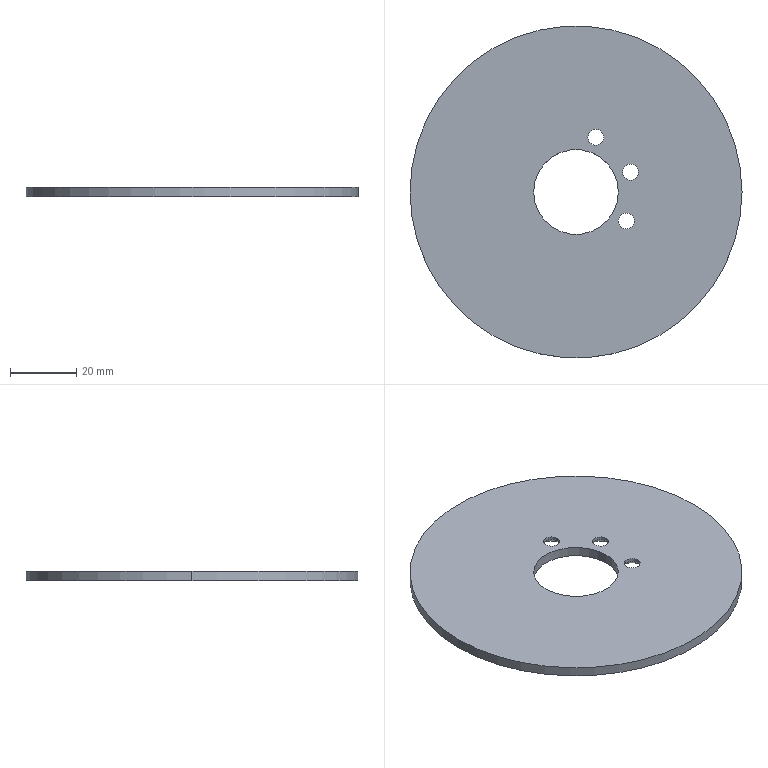Part | SolidWorks | features Extrusion 1, HoleWzd 1 | 1 solid | 18 faces | box 100 x 100 x 3 mm | volume 21741 mm3 | cylinder 10 | cone 6 | plane 2 | commonest cylinder face diameters 4.8 x6 25.5 x2 100 x2
STEP:
#1=CARTESIAN_POINT('',(8.385,16.445,2.08));
#2=VERTEX_POINT('',#1);
#3=CARTESIAN_POINT('',(3.585,16.445,2.08));
#4=VERTEX_POINT('',#3);
#5=CARTESIAN_POINT('',(5.985,16.445,2.08));
#6=DIRECTION('',(0.,0.,-1.));
#7=DIRECTION('',(-1.,0.,0.));
#8=AXIS2_PLACEMENT_3D('',#5,#6,#7);
#9=CIRCLE('',#8,2.4);
#10=EDGE_CURVE('',#2,#4,#9,.T.);
#11=ORIENTED_EDGE('',*,*,#10,.F.);
#12=CARTESIAN_POINT('',(10.465,16.445,0.));
#13=VERTEX_POINT('',#12);
#14=CARTESIAN_POINT('',(10.465,16.445,0.));
#15=DIRECTION('',(0.7071,0.,-0.7071));
#16=VECTOR('',#15,1000.);
#17=LINE('',#14,#16);
#18=EDGE_CURVE('',#2,#13,#17,.T.);
#19=ORIENTED_EDGE('',*,*,#18,.T.);
#20=CARTESIAN_POINT('',(1.505,16.445,0.));
#21=VERTEX_POINT('',#20);
#22=CARTESIAN_POINT('',(5.985,16.445,0.));
#23=DIRECTION('',(0.,0.,-1.));
#24=DIRECTION('',(-1.,0.,0.));
#25=AXIS2_PLACEMENT_3D('',#22,#23,#24);
#26=CIRCLE('',#25,4.48);
#27=EDGE_CURVE('',#13,#21,#26,.T.);
#28=ORIENTED_EDGE('',*,*,#27,.T.);
#29=CARTESIAN_POINT('',(1.505,16.445,0.));
#30=DIRECTION('',(-0.7071,0.,-0.7071));
#31=VECTOR('',#30,1000.);
#32=LINE('',#29,#31);
#33=EDGE_CURVE('',#4,#21,#32,.T.);
#34=ORIENTED_EDGE('',*,*,#33,.F.);
#35=EDGE_LOOP('',(#11,#19,#28,#34));
#36=FACE_OUTER_BOUND('',#35,.T.);
#37=CARTESIAN_POINT('',(5.985,16.445,0.));
#38=DIRECTION('',(0.,0.,-1.));
#39=DIRECTION('',(-1.,0.,0.));
#40=AXIS2_PLACEMENT_3D('',#37,#38,#39);
#41=CONICAL_SURFACE('',#40,4.48,0.7854);
#42=ADVANCED_FACE('',(#36),#41,.F.);
#43=CARTESIAN_POINT('',(8.385,16.445,3.));
#44=VERTEX_POINT('',#43);
#45=CARTESIAN_POINT('',(3.585,16.445,3.));
#46=VERTEX_POINT('',#45);
#47=CARTESIAN_POINT('',(5.985,16.445,3.));
#48=DIRECTION('',(0.,0.,-1.));
#49=DIRECTION('',(-1.,0.,0.));
#50=AXIS2_PLACEMENT_3D('',#47,#48,#49);
#51=CIRCLE('',#50,2.4);
#52=EDGE_CURVE('',#44,#46,#51,.T.);
#53=ORIENTED_EDGE('',*,*,#52,.F.);
#54=CARTESIAN_POINT('',(8.385,16.445,0.));
#55=DIRECTION('',(0.,0.,-1.));
#56=VECTOR('',#55,1000.);
#57=LINE('',#54,#56);
#58=EDGE_CURVE('',#44,#2,#57,.T.);
#59=ORIENTED_EDGE('',*,*,#58,.T.);
#60=ORIENTED_EDGE('',*,*,#10,.T.);
#61=CARTESIAN_POINT('',(3.585,16.445,0.));
#62=DIRECTION('',(0.,0.,-1.));
#63=VECTOR('',#62,1000.);
#64=LINE('',#61,#63);
#65=EDGE_CURVE('',#46,#4,#64,.T.);
#66=ORIENTED_EDGE('',*,*,#65,.F.);
#67=EDGE_LOOP('',(#53,#59,#60,#66));
#68=FACE_OUTER_BOUND('',#67,.T.);
#69=CARTESIAN_POINT('',(5.985,16.445,0.));
#70=DIRECTION('',(0.,0.,-1.));
#71=DIRECTION('',(-1.,0.,0.));
#72=AXIS2_PLACEMENT_3D('',#69,#70,#71);
#73=CYLINDRICAL_SURFACE('',#72,2.4);
#74=ADVANCED_FACE('',(#68),#73,.F.);
#75=CARTESIAN_POINT('',(17.555,-8.75,2.08));
#76=VERTEX_POINT('',#75);
#77=CARTESIAN_POINT('',(12.755,-8.75,2.08));
#78=VERTEX_POINT('',#77);
#79=CARTESIAN_POINT('',(15.155,-8.75,2.08));
#80=DIRECTION('',(0.,0.,-1.));
#81=DIRECTION('',(-1.,0.,0.));
#82=AXIS2_PLACEMENT_3D('',#79,#80,#81);
#83=CIRCLE('',#82,2.4);
#84=EDGE_CURVE('',#76,#78,#83,.T.);
#85=ORIENTED_EDGE('',*,*,#84,.F.);
#86=CARTESIAN_POINT('',(19.635,-8.75,0.));
#87=VERTEX_POINT('',#86);
#88=CARTESIAN_POINT('',(19.635,-8.75,0.));
#89=DIRECTION('',(0.7071,0.,-0.7071));
#90=VECTOR('',#89,1000.);
#91=LINE('',#88,#90);
#92=EDGE_CURVE('',#76,#87,#91,.T.);
#93=ORIENTED_EDGE('',*,*,#92,.T.);
#94=CARTESIAN_POINT('',(10.675,-8.75,0.));
#95=VERTEX_POINT('',#94);
#96=CARTESIAN_POINT('',(15.155,-8.75,0.));
#97=DIRECTION('',(0.,0.,-1.));
#98=DIRECTION('',(-1.,0.,0.));
#99=AXIS2_PLACEMENT_3D('',#96,#97,#98);
#100=CIRCLE('',#99,4.48);
#101=EDGE_CURVE('',#87,#95,#100,.T.);
#102=ORIENTED_EDGE('',*,*,#101,.T.);
#103=CARTESIAN_POINT('',(10.675,-8.75,0.));
#104=DIRECTION('',(-0.7071,0.,-0.7071));
#105=VECTOR('',#104,1000.);
#106=LINE('',#103,#105);
#107=EDGE_CURVE('',#78,#95,#106,.T.);
#108=ORIENTED_EDGE('',*,*,#107,.F.);
#109=EDGE_LOOP('',(#85,#93,#102,#108));
#110=FACE_OUTER_BOUND('',#109,.T.);
#111=CARTESIAN_POINT('',(15.155,-8.75,0.));
#112=DIRECTION('',(0.,0.,-1.));
#113=DIRECTION('',(-1.,0.,0.));
#114=AXIS2_PLACEMENT_3D('',#111,#112,#113);
#115=CONICAL_SURFACE('',#114,4.48,0.7854);
#116=ADVANCED_FACE('',(#110),#115,.F.);
#117=CARTESIAN_POINT('',(17.555,-8.75,3.));
#118=VERTEX_POINT('',#117);
#119=CARTESIAN_POINT('',(12.755,-8.75,3.));
#120=VERTEX_POINT('',#119);
#121=CARTESIAN_POINT('',(15.155,-8.75,3.));
#122=DIRECTION('',(0.,0.,-1.));
#123=DIRECTION('',(-1.,0.,0.));
#124=AXIS2_PLACEMENT_3D('',#121,#122,#123);
#125=CIRCLE('',#124,2.4);
#126=EDGE_CURVE('',#118,#120,#125,.T.);
#127=ORIENTED_EDGE('',*,*,#126,.F.);
#128=CARTESIAN_POINT('',(17.555,-8.75,0.));
#129=DIRECTION('',(0.,0.,-1.));
#130=VECTOR('',#129,1000.);
#131=LINE('',#128,#130);
#132=EDGE_CURVE('',#118,#76,#131,.T.);
#133=ORIENTED_EDGE('',*,*,#132,.T.);
#134=ORIENTED_EDGE('',*,*,#84,.T.);
#135=CARTESIAN_POINT('',(12.755,-8.75,0.));
#136=DIRECTION('',(0.,0.,-1.));
#137=VECTOR('',#136,1000.);
#138=LINE('',#135,#137);
#139=EDGE_CURVE('',#120,#78,#138,.T.);
#140=ORIENTED_EDGE('',*,*,#139,.F.);
#141=EDGE_LOOP('',(#127,#133,#134,#140));
#142=FACE_OUTER_BOUND('',#141,.T.);
#143=CARTESIAN_POINT('',(15.155,-8.75,0.));
#144=DIRECTION('',(0.,0.,-1.));
#145=DIRECTION('',(-1.,0.,0.));
#146=AXIS2_PLACEMENT_3D('',#143,#144,#145);
#147=CYLINDRICAL_SURFACE('',#146,2.4);
#148=ADVANCED_FACE('',(#142),#147,.F.);
#149=CARTESIAN_POINT('',(18.845,5.985,2.08));
#150=VERTEX_POINT('',#149);
#151=CARTESIAN_POINT('',(14.045,5.985,2.08));
#152=VERTEX_POINT('',#151);
#153=CARTESIAN_POINT('',(16.445,5.985,2.08));
#154=DIRECTION('',(0.,0.,-1.));
#155=DIRECTION('',(-1.,0.,0.));
#156=AXIS2_PLACEMENT_3D('',#153,#154,#155);
#157=CIRCLE('',#156,2.4);
#158=EDGE_CURVE('',#150,#152,#157,.T.);
#159=ORIENTED_EDGE('',*,*,#158,.F.);
#160=CARTESIAN_POINT('',(20.925,5.985,0.));
#161=VERTEX_POINT('',#160);
#162=CARTESIAN_POINT('',(20.925,5.985,0.));
#163=DIRECTION('',(0.7071,0.,-0.7071));
#164=VECTOR('',#163,1000.);
#165=LINE('',#162,#164);
#166=EDGE_CURVE('',#150,#161,#165,.T.);
#167=ORIENTED_EDGE('',*,*,#166,.T.);
#168=CARTESIAN_POINT('',(11.965,5.985,0.));
#169=VERTEX_POINT('',#168);
#170=CARTESIAN_POINT('',(16.445,5.985,0.));
#171=DIRECTION('',(0.,0.,-1.));
#172=DIRECTION('',(-1.,0.,0.));
#173=AXIS2_PLACEMENT_3D('',#170,#171,#172);
#174=CIRCLE('',#173,4.48);
#175=EDGE_CURVE('',#161,#169,#174,.T.);
#176=ORIENTED_EDGE('',*,*,#175,.T.);
#177=CARTESIAN_POINT('',(11.965,5.985,0.));
#178=DIRECTION('',(-0.7071,0.,-0.7071));
#179=VECTOR('',#178,1000.);
#180=LINE('',#177,#179);
#181=EDGE_CURVE('',#152,#169,#180,.T.);
#182=ORIENTED_EDGE('',*,*,#181,.F.);
#183=EDGE_LOOP('',(#159,#167,#176,#182));
#184=FACE_OUTER_BOUND('',#183,.T.);
#185=CARTESIAN_POINT('',(16.445,5.985,0.));
#186=DIRECTION('',(0.,0.,-1.));
#187=DIRECTION('',(-1.,0.,0.));
#188=AXIS2_PLACEMENT_3D('',#185,#186,#187);
#189=CONICAL_SURFACE('',#188,4.48,0.7854);
#190=ADVANCED_FACE('',(#184),#189,.F.);
#191=CARTESIAN_POINT('',(18.845,5.985,3.));
#192=VERTEX_POINT('',#191);
#193=CARTESIAN_POINT('',(14.045,5.985,3.));
#194=VERTEX_POINT('',#193);
#195=CARTESIAN_POINT('',(16.445,5.985,3.));
#196=DIRECTION('',(0.,0.,-1.));
#197=DIRECTION('',(-1.,0.,0.));
#198=AXIS2_PLACEMENT_3D('',#195,#196,#197);
#199=CIRCLE('',#198,2.4);
#200=EDGE_CURVE('',#192,#194,#199,.T.);
#201=ORIENTED_EDGE('',*,*,#200,.F.);
#202=CARTESIAN_POINT('',(18.845,5.985,0.));
#203=DIRECTION('',(0.,0.,-1.));
#204=VECTOR('',#203,1000.);
#205=LINE('',#202,#204);
#206=EDGE_CURVE('',#192,#150,#205,.T.);
#207=ORIENTED_EDGE('',*,*,#206,.T.);
#208=ORIENTED_EDGE('',*,*,#158,.T.);
#209=CARTESIAN_POINT('',(14.045,5.985,0.));
#210=DIRECTION('',(0.,0.,-1.));
#211=VECTOR('',#210,1000.);
#212=LINE('',#209,#211);
#213=EDGE_CURVE('',#194,#152,#212,.T.);
#214=ORIENTED_EDGE('',*,*,#213,.F.);
#215=EDGE_LOOP('',(#201,#207,#208,#214));
#216=FACE_OUTER_BOUND('',#215,.T.);
#217=CARTESIAN_POINT('',(16.445,5.985,0.));
#218=DIRECTION('',(0.,0.,-1.));
#219=DIRECTION('',(-1.,0.,0.));
#220=AXIS2_PLACEMENT_3D('',#217,#218,#219);
#221=CYLINDRICAL_SURFACE('',#220,2.4);
#222=ADVANCED_FACE('',(#216),#221,.F.);
#223=CARTESIAN_POINT('',(-12.75,0.,3.));
#224=VERTEX_POINT('',#223);
#225=CARTESIAN_POINT('',(12.75,0.,3.));
#226=VERTEX_POINT('',#225);
#227=CARTESIAN_POINT('',(0.,0.,3.));
#228=DIRECTION('',(0.,0.,1.));
#229=DIRECTION('',(1.,0.,0.));
#230=AXIS2_PLACEMENT_3D('',#227,#228,#229);
#231=CIRCLE('',#230,12.75);
#232=EDGE_CURVE('',#224,#226,#231,.T.);
#233=ORIENTED_EDGE('',*,*,#232,.T.);
#234=CARTESIAN_POINT('',(12.75,0.,0.));
#235=VERTEX_POINT('',#234);
#236=CARTESIAN_POINT('',(12.75,0.,3.));
#237=DIRECTION('',(0.,0.,-1.));
#238=VECTOR('',#237,1000.);
#239=LINE('',#236,#238);
#240=EDGE_CURVE('',#226,#235,#239,.T.);
#241=ORIENTED_EDGE('',*,*,#240,.T.);
#242=CARTESIAN_POINT('',(-12.75,0.,0.));
#243=VERTEX_POINT('',#242);
#244=CARTESIAN_POINT('',(0.,0.,0.));
#245=DIRECTION('',(0.,0.,1.));
#246=DIRECTION('',(1.,0.,0.));
#247=AXIS2_PLACEMENT_3D('',#244,#245,#246);
#248=CIRCLE('',#247,12.75);
#249=EDGE_CURVE('',#243,#235,#248,.T.);
#250=ORIENTED_EDGE('',*,*,#249,.F.);
#251=CARTESIAN_POINT('',(-12.75,0.,3.));
#252=DIRECTION('',(0.,0.,-1.));
#253=VECTOR('',#252,1000.);
#254=LINE('',#251,#253);
#255=EDGE_CURVE('',#224,#243,#254,.T.);
#256=ORIENTED_EDGE('',*,*,#255,.F.);
#257=EDGE_LOOP('',(#233,#241,#250,#256));
#258=FACE_OUTER_BOUND('',#257,.T.);
#259=CARTESIAN_POINT('',(0.,0.,3.));
#260=DIRECTION('',(0.,0.,-1.));
#261=DIRECTION('',(-1.,0.,0.));
#262=AXIS2_PLACEMENT_3D('',#259,#260,#261);
#263=CYLINDRICAL_SURFACE('',#262,12.75);
#264=ADVANCED_FACE('',(#258),#263,.F.);
#265=CARTESIAN_POINT('',(50.,0.,3.));
#266=VERTEX_POINT('',#265);
#267=CARTESIAN_POINT('',(-50.,0.,3.));
#268=VERTEX_POINT('',#267);
#269=CARTESIAN_POINT('',(0.,0.,3.));
#270=DIRECTION('',(0.,0.,1.));
#271=DIRECTION('',(1.,0.,0.));
#272=AXIS2_PLACEMENT_3D('',#269,#270,#271);
#273=CIRCLE('',#272,50.);
#274=EDGE_CURVE('',#266,#268,#273,.T.);
#275=ORIENTED_EDGE('',*,*,#274,.F.);
#276=CARTESIAN_POINT('',(50.,0.,0.));
#277=VERTEX_POINT('',#276);
#278=CARTESIAN_POINT('',(50.,0.,3.));
#279=DIRECTION('',(0.,0.,-1.));
#280=VECTOR('',#279,1000.);
#281=LINE('',#278,#280);
#282=EDGE_CURVE('',#266,#277,#281,.T.);
#283=ORIENTED_EDGE('',*,*,#282,.T.);
#284=CARTESIAN_POINT('',(-50.,0.,0.));
#285=VERTEX_POINT('',#284);
#286=CARTESIAN_POINT('',(0.,0.,0.));
#287=DIRECTION('',(0.,0.,1.));
#288=DIRECTION('',(1.,0.,0.));
#289=AXIS2_PLACEMENT_3D('',#286,#287,#288);
#290=CIRCLE('',#289,50.);
#291=EDGE_CURVE('',#277,#285,#290,.T.);
#292=ORIENTED_EDGE('',*,*,#291,.T.);
#293=CARTESIAN_POINT('',(-50.,0.,3.));
#294=DIRECTION('',(0.,0.,-1.));
#295=VECTOR('',#294,1000.);
#296=LINE('',#293,#295);
#297=EDGE_CURVE('',#268,#285,#296,.T.);
#298=ORIENTED_EDGE('',*,*,#297,.F.);
#299=EDGE_LOOP('',(#275,#283,#292,#298));
#300=FACE_OUTER_BOUND('',#299,.T.);
#301=CARTESIAN_POINT('',(0.,0.,3.));
#302=DIRECTION('',(0.,0.,-1.));
#303=DIRECTION('',(-1.,0.,0.));
#304=AXIS2_PLACEMENT_3D('',#301,#302,#303);
#305=CYLINDRICAL_SURFACE('',#304,50.);
#306=ADVANCED_FACE('',(#300),#305,.T.);
#307=CARTESIAN_POINT('',(5.985,16.445,3.));
#308=DIRECTION('',(0.,0.,-1.));
#309=DIRECTION('',(-1.,0.,0.));
#310=AXIS2_PLACEMENT_3D('',#307,#308,#309);
#311=CIRCLE('',#310,2.4);
#312=EDGE_CURVE('',#46,#44,#311,.T.);
#313=ORIENTED_EDGE('',*,*,#312,.T.);
#314=ORIENTED_EDGE('',*,*,#52,.T.);
#315=EDGE_LOOP('',(#313,#314));
#316=FACE_BOUND('',#315,.T.);
#317=CARTESIAN_POINT('',(15.155,-8.75,3.));
#318=DIRECTION('',(0.,0.,-1.));
#319=DIRECTION('',(-1.,0.,0.));
#320=AXIS2_PLACEMENT_3D('',#317,#318,#319);
#321=CIRCLE('',#320,2.4);
#322=EDGE_CURVE('',#120,#118,#321,.T.);
#323=ORIENTED_EDGE('',*,*,#322,.T.);
#324=ORIENTED_EDGE('',*,*,#126,.T.);
#325=EDGE_LOOP('',(#323,#324));
#326=FACE_BOUND('',#325,.T.);
#327=CARTESIAN_POINT('',(16.445,5.985,3.));
#328=DIRECTION('',(0.,0.,-1.));
#329=DIRECTION('',(-1.,0.,0.));
#330=AXIS2_PLACEMENT_3D('',#327,#328,#329);
#331=CIRCLE('',#330,2.4);
#332=EDGE_CURVE('',#194,#192,#331,.T.);
#333=ORIENTED_EDGE('',*,*,#332,.T.);
#334=ORIENTED_EDGE('',*,*,#200,.T.);
#335=EDGE_LOOP('',(#333,#334));
#336=FACE_BOUND('',#335,.T.);
#337=CARTESIAN_POINT('',(0.,0.,3.));
#338=DIRECTION('',(0.,0.,1.));
#339=DIRECTION('',(1.,0.,0.));
#340=AXIS2_PLACEMENT_3D('',#337,#338,#339);
#341=CIRCLE('',#340,50.);
#342=EDGE_CURVE('',#268,#266,#341,.T.);
#343=ORIENTED_EDGE('',*,*,#342,.T.);
#344=ORIENTED_EDGE('',*,*,#274,.T.);
#345=EDGE_LOOP('',(#343,#344));
#346=FACE_OUTER_BOUND('',#345,.T.);
#347=ORIENTED_EDGE('',*,*,#232,.F.);
#348=CARTESIAN_POINT('',(0.,0.,3.));
#349=DIRECTION('',(0.,0.,1.));
#350=DIRECTION('',(1.,0.,0.));
#351=AXIS2_PLACEMENT_3D('',#348,#349,#350);
#352=CIRCLE('',#351,12.75);
#353=EDGE_CURVE('',#226,#224,#352,.T.);
#354=ORIENTED_EDGE('',*,*,#353,.F.);
#355=EDGE_LOOP('',(#347,#354));
#356=FACE_BOUND('',#355,.T.);
#357=CARTESIAN_POINT('',(0.,0.,3.));
#358=DIRECTION('',(0.,0.,1.));
#359=DIRECTION('',(1.,0.,0.));
#360=AXIS2_PLACEMENT_3D('',#357,#358,#359);
#361=PLANE('',#360);
#362=ADVANCED_FACE('',(#316,#326,#336,#346,#356),#361,.T.);
#363=CARTESIAN_POINT('',(5.985,16.445,0.));
#364=DIRECTION('',(0.,0.,-1.));
#365=DIRECTION('',(-1.,0.,0.));
#366=AXIS2_PLACEMENT_3D('',#363,#364,#365);
#367=CIRCLE('',#366,4.48);
#368=EDGE_CURVE('',#21,#13,#367,.T.);
#369=ORIENTED_EDGE('',*,*,#368,.F.);
#370=ORIENTED_EDGE('',*,*,#27,.F.);
#371=EDGE_LOOP('',(#369,#370));
#372=FACE_BOUND('',#371,.T.);
#373=CARTESIAN_POINT('',(15.155,-8.75,0.));
#374=DIRECTION('',(0.,0.,-1.));
#375=DIRECTION('',(-1.,0.,0.));
#376=AXIS2_PLACEMENT_3D('',#373,#374,#375);
#377=CIRCLE('',#376,4.48);
#378=EDGE_CURVE('',#95,#87,#377,.T.);
#379=ORIENTED_EDGE('',*,*,#378,.F.);
#380=ORIENTED_EDGE('',*,*,#101,.F.);
#381=EDGE_LOOP('',(#379,#380));
#382=FACE_BOUND('',#381,.T.);
#383=CARTESIAN_POINT('',(16.445,5.985,0.));
#384=DIRECTION('',(0.,0.,-1.));
#385=DIRECTION('',(-1.,0.,0.));
#386=AXIS2_PLACEMENT_3D('',#383,#384,#385);
#387=CIRCLE('',#386,4.48);
#388=EDGE_CURVE('',#169,#161,#387,.T.);
#389=ORIENTED_EDGE('',*,*,#388,.F.);
#390=ORIENTED_EDGE('',*,*,#175,.F.);
#391=EDGE_LOOP('',(#389,#390));
#392=FACE_BOUND('',#391,.T.);
#393=CARTESIAN_POINT('',(0.,0.,0.));
#394=DIRECTION('',(0.,0.,1.));
#395=DIRECTION('',(1.,0.,0.));
#396=AXIS2_PLACEMENT_3D('',#393,#394,#395);
#397=CIRCLE('',#396,50.);
#398=EDGE_CURVE('',#285,#277,#397,.T.);
#399=ORIENTED_EDGE('',*,*,#398,.F.);
#400=ORIENTED_EDGE('',*,*,#291,.F.);
#401=EDGE_LOOP('',(#399,#400));
#402=FACE_OUTER_BOUND('',#401,.T.);
#403=ORIENTED_EDGE('',*,*,#249,.T.);
#404=CARTESIAN_POINT('',(0.,0.,0.));
#405=DIRECTION('',(0.,0.,1.));
#406=DIRECTION('',(1.,0.,0.));
#407=AXIS2_PLACEMENT_3D('',#404,#405,#406);
#408=CIRCLE('',#407,12.75);
#409=EDGE_CURVE('',#235,#243,#408,.T.);
#410=ORIENTED_EDGE('',*,*,#409,.T.);
#411=EDGE_LOOP('',(#403,#410));
#412=FACE_BOUND('',#411,.T.);
#413=CARTESIAN_POINT('',(0.,0.,0.));
#414=DIRECTION('',(0.,0.,1.));
#415=DIRECTION('',(1.,0.,0.));
#416=AXIS2_PLACEMENT_3D('',#413,#414,#415);
#417=PLANE('',#416);
#418=ADVANCED_FACE('',(#372,#382,#392,#402,#412),#417,.F.);
#419=ORIENTED_EDGE('',*,*,#282,.F.);
#420=ORIENTED_EDGE('',*,*,#342,.F.);
#421=ORIENTED_EDGE('',*,*,#297,.T.);
#422=ORIENTED_EDGE('',*,*,#398,.T.);
#423=EDGE_LOOP('',(#419,#420,#421,#422));
#424=FACE_OUTER_BOUND('',#423,.T.);
#425=CARTESIAN_POINT('',(0.,0.,3.));
#426=DIRECTION('',(0.,0.,-1.));
#427=DIRECTION('',(-1.,0.,0.));
#428=AXIS2_PLACEMENT_3D('',#425,#426,#427);
#429=CYLINDRICAL_SURFACE('',#428,50.);
#430=ADVANCED_FACE('',(#424),#429,.T.);
#431=ORIENTED_EDGE('',*,*,#240,.F.);
#432=ORIENTED_EDGE('',*,*,#353,.T.);
#433=ORIENTED_EDGE('',*,*,#255,.T.);
#434=ORIENTED_EDGE('',*,*,#409,.F.);
#435=EDGE_LOOP('',(#431,#432,#433,#434));
#436=FACE_OUTER_BOUND('',#435,.T.);
#437=CARTESIAN_POINT('',(0.,0.,3.));
#438=DIRECTION('',(0.,0.,-1.));
#439=DIRECTION('',(-1.,0.,0.));
#440=AXIS2_PLACEMENT_3D('',#437,#438,#439);
#441=CYLINDRICAL_SURFACE('',#440,12.75);
#442=ADVANCED_FACE('',(#436),#441,.F.);
#443=ORIENTED_EDGE('',*,*,#206,.F.);
#444=ORIENTED_EDGE('',*,*,#332,.F.);
#445=ORIENTED_EDGE('',*,*,#213,.T.);
#446=CARTESIAN_POINT('',(16.445,5.985,2.08));
#447=DIRECTION('',(0.,0.,-1.));
#448=DIRECTION('',(-1.,0.,0.));
#449=AXIS2_PLACEMENT_3D('',#446,#447,#448);
#450=CIRCLE('',#449,2.4);
#451=EDGE_CURVE('',#152,#150,#450,.T.);
#452=ORIENTED_EDGE('',*,*,#451,.T.);
#453=EDGE_LOOP('',(#443,#444,#445,#452));
#454=FACE_OUTER_BOUND('',#453,.T.);
#455=CARTESIAN_POINT('',(16.445,5.985,0.));
#456=DIRECTION('',(0.,0.,-1.));
#457=DIRECTION('',(-1.,0.,0.));
#458=AXIS2_PLACEMENT_3D('',#455,#456,#457);
#459=CYLINDRICAL_SURFACE('',#458,2.4);
#460=ADVANCED_FACE('',(#454),#459,.F.);
#461=ORIENTED_EDGE('',*,*,#166,.F.);
#462=ORIENTED_EDGE('',*,*,#451,.F.);
#463=ORIENTED_EDGE('',*,*,#181,.T.);
#464=ORIENTED_EDGE('',*,*,#388,.T.);
#465=EDGE_LOOP('',(#461,#462,#463,#464));
#466=FACE_OUTER_BOUND('',#465,.T.);
#467=CARTESIAN_POINT('',(16.445,5.985,0.));
#468=DIRECTION('',(0.,0.,-1.));
#469=DIRECTION('',(-1.,0.,0.));
#470=AXIS2_PLACEMENT_3D('',#467,#468,#469);
#471=CONICAL_SURFACE('',#470,4.48,0.7854);
#472=ADVANCED_FACE('',(#466),#471,.F.);
#473=ORIENTED_EDGE('',*,*,#132,.F.);
#474=ORIENTED_EDGE('',*,*,#322,.F.);
#475=ORIENTED_EDGE('',*,*,#139,.T.);
#476=CARTESIAN_POINT('',(15.155,-8.75,2.08));
#477=DIRECTION('',(0.,0.,-1.));
#478=DIRECTION('',(-1.,0.,0.));
#479=AXIS2_PLACEMENT_3D('',#476,#477,#478);
#480=CIRCLE('',#479,2.4);
#481=EDGE_CURVE('',#78,#76,#480,.T.);
#482=ORIENTED_EDGE('',*,*,#481,.T.);
#483=EDGE_LOOP('',(#473,#474,#475,#482));
#484=FACE_OUTER_BOUND('',#483,.T.);
#485=CARTESIAN_POINT('',(15.155,-8.75,0.));
#486=DIRECTION('',(0.,0.,-1.));
#487=DIRECTION('',(-1.,0.,0.));
#488=AXIS2_PLACEMENT_3D('',#485,#486,#487);
#489=CYLINDRICAL_SURFACE('',#488,2.4);
#490=ADVANCED_FACE('',(#484),#489,.F.);
#491=ORIENTED_EDGE('',*,*,#92,.F.);
#492=ORIENTED_EDGE('',*,*,#481,.F.);
#493=ORIENTED_EDGE('',*,*,#107,.T.);
#494=ORIENTED_EDGE('',*,*,#378,.T.);
#495=EDGE_LOOP('',(#491,#492,#493,#494));
#496=FACE_OUTER_BOUND('',#495,.T.);
#497=CARTESIAN_POINT('',(15.155,-8.75,0.));
#498=DIRECTION('',(0.,0.,-1.));
#499=DIRECTION('',(-1.,0.,0.));
#500=AXIS2_PLACEMENT_3D('',#497,#498,#499);
#501=CONICAL_SURFACE('',#500,4.48,0.7854);
#502=ADVANCED_FACE('',(#496),#501,.F.);
#503=ORIENTED_EDGE('',*,*,#58,.F.);
#504=ORIENTED_EDGE('',*,*,#312,.F.);
#505=ORIENTED_EDGE('',*,*,#65,.T.);
#506=CARTESIAN_POINT('',(5.985,16.445,2.08));
#507=DIRECTION('',(0.,0.,-1.));
#508=DIRECTION('',(-1.,0.,0.));
#509=AXIS2_PLACEMENT_3D('',#506,#507,#508);
#510=CIRCLE('',#509,2.4);
#511=EDGE_CURVE('',#4,#2,#510,.T.);
#512=ORIENTED_EDGE('',*,*,#511,.T.);
#513=EDGE_LOOP('',(#503,#504,#505,#512));
#514=FACE_OUTER_BOUND('',#513,.T.);
#515=CARTESIAN_POINT('',(5.985,16.445,0.));
#516=DIRECTION('',(0.,0.,-1.));
#517=DIRECTION('',(-1.,0.,0.));
#518=AXIS2_PLACEMENT_3D('',#515,#516,#517);
#519=CYLINDRICAL_SURFACE('',#518,2.4);
#520=ADVANCED_FACE('',(#514),#519,.F.);
#521=ORIENTED_EDGE('',*,*,#18,.F.);
#522=ORIENTED_EDGE('',*,*,#511,.F.);
#523=ORIENTED_EDGE('',*,*,#33,.T.);
#524=ORIENTED_EDGE('',*,*,#368,.T.);
#525=EDGE_LOOP('',(#521,#522,#523,#524));
#526=FACE_OUTER_BOUND('',#525,.T.);
#527=CARTESIAN_POINT('',(5.985,16.445,0.));
#528=DIRECTION('',(0.,0.,-1.));
#529=DIRECTION('',(-1.,0.,0.));
#530=AXIS2_PLACEMENT_3D('',#527,#528,#529);
#531=CONICAL_SURFACE('',#530,4.48,0.7854);
#532=ADVANCED_FACE('',(#526),#531,.F.);
#533=CLOSED_SHELL('',(#42,#74,#116,#148,#190,#222,#264,#306,#362,#418,#430,#442,#460,#472,#490,#502,#520,#532));
#534=MANIFOLD_SOLID_BREP('',#533);
#535=CARTESIAN_POINT('',(0.,0.,0.));
#536=DIRECTION('',(0.,0.,1.));
#537=DIRECTION('',(1.,0.,0.));
#538=AXIS2_PLACEMENT_3D('',#535,#536,#537);
#539=(LENGTH_UNIT()NAMED_UNIT(*)SI_UNIT(.MILLI.,.METRE.));
#540=UNCERTAINTY_MEASURE_WITH_UNIT(LENGTH_MEASURE(0.00001),#539,'','');
#541=(NAMED_UNIT(*)PLANE_ANGLE_UNIT()SI_UNIT($,.RADIAN.));
#542=(NAMED_UNIT(*)SI_UNIT($,.STERADIAN.)SOLID_ANGLE_UNIT());
#543=(GEOMETRIC_REPRESENTATION_CONTEXT(3)GLOBAL_UNCERTAINTY_ASSIGNED_CONTEXT((#540))GLOBAL_UNIT_ASSIGNED_CONTEXT((#539,#541,#542))REPRESENTATION_CONTEXT('',''));
#544=ADVANCED_BREP_SHAPE_REPRESENTATION('',(#534,#538),#543);